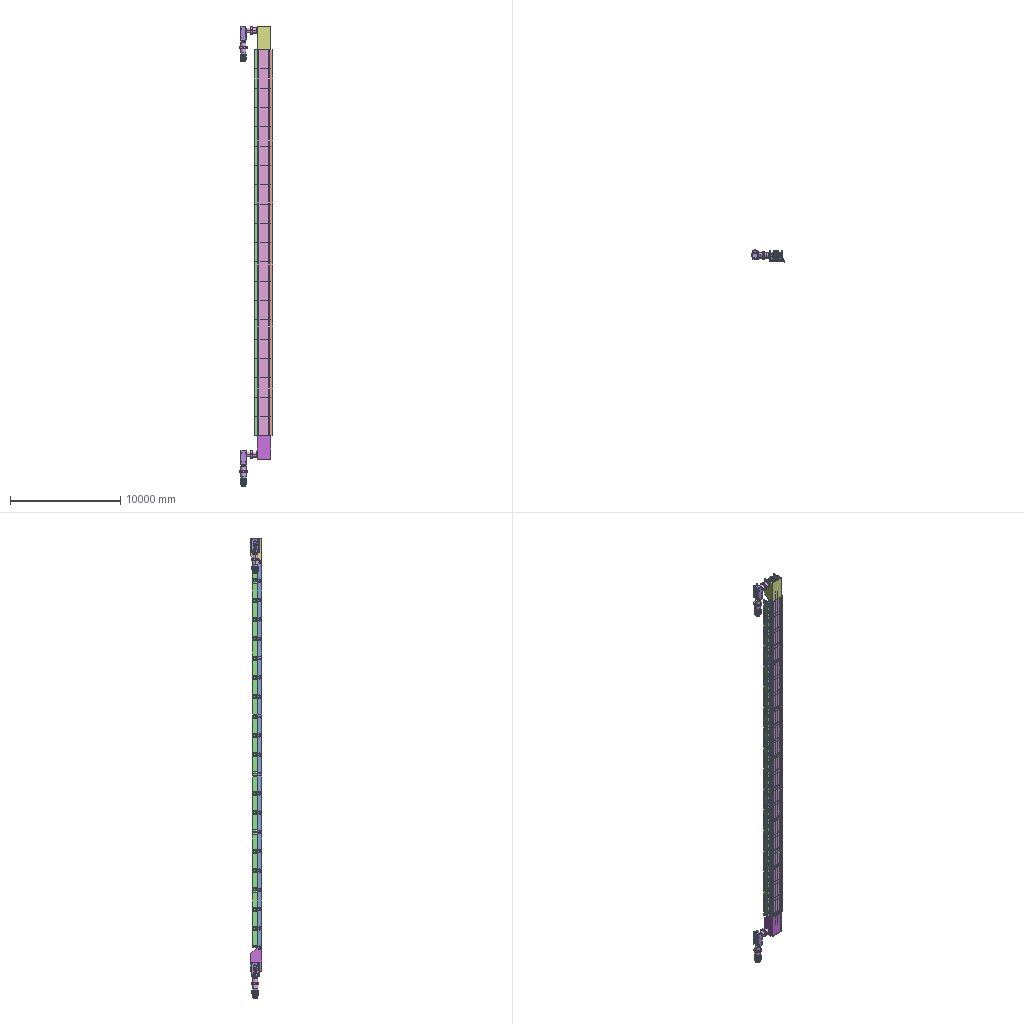Assembly | SolidWorks | 41 different items | 1422 placed | box 2996 x 1048 x 41686 mm
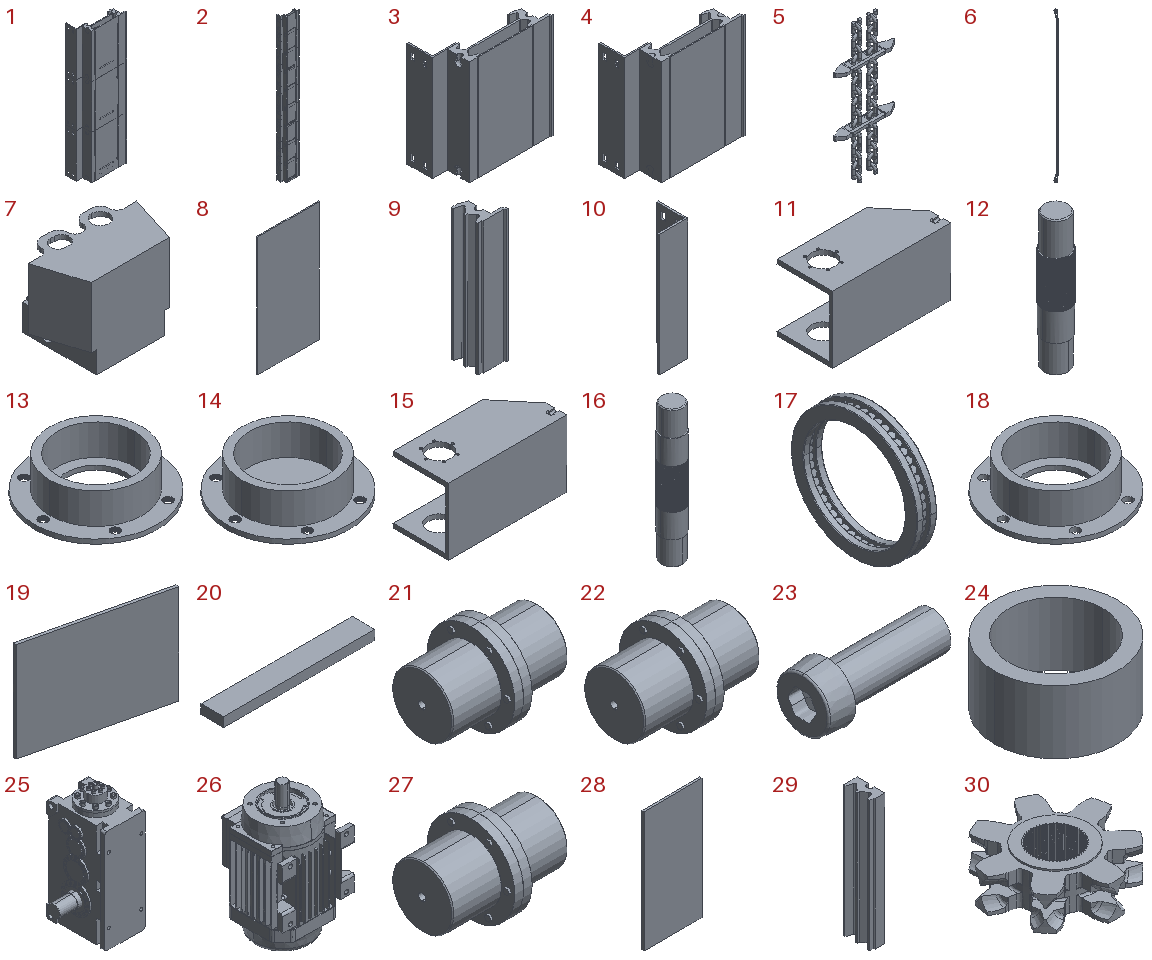Parts list (item | name | quantity | parent item | size | volume | features):
1 | (subassembly) | x6 | in 2 | 1628 x 811.488 x 5250 mm | 1041325350 mm3 | -
2 | (subassembly) | x2 | - | - | 3123900816 mm3 | -
3 | (subassembly) | x1 | - | 1628 x 811.488 x 1750 mm | 332107465 mm3 | -
4 | (subassembly) | x20 | in 1 | 1628 x 811.488 x 1750 mm | 345627340 mm3 | -
5 | (subassembly) | x1 | - | 984.376 x 173.983 x 2274 mm | 39316055 mm3 | features ReferencePattern 36, Cut 1, LocalChainPattern 1
6 | (subassembly) | x2 | - | - | 584235551 mm3 | features ReferencePattern 518, RefAxis 2, LocalChainPattern 1
7 | - | x40 | in 4 | 498.198 x 340 x 380 mm | 18859661 mm3 | features ICE 7, 3DProfileFeature 6, BlendCut 1, Extrusion 1, MirrorPattern 1
8 | - | x20 | in 4 | 903 x 15 x 1750 mm | 23703750 mm3 | features Extrusion 1
9 | - | x20 | in 4 | 368.945 x 388.507 x 1750 mm | 104894918 mm3 | features 3DProfileFeature 2, ICE 2, Extrusion 1, MirrorPattern 1, RevCut 1
10 | - | x20 | in 4 | 410 x 422.981 x 1750 mm | 34749166 mm3 | features Extrusion 1, ICE 1
11 | - | x1 | - | 2125 x 1000 x 1200 mm | 401885685 mm3 | features ICE 6, 3DProfileFeature 4, MirrorPattern 4, Extrusion 1, RevCut 1
12 | - | x1 | - | 294.723 x 294.709 x 1450 mm | 87344155 mm3 | features ICE 5, 3DProfileFeature 1, Chamfer 1, CirPattern 1, Extrusion 1, Fillet 1
13 | - | x1 | - | 560 x 560 x 160 mm | 9604413 mm3 | features SweepThread 6, ICE 4, 3DProfileFeature 1, Extrusion 1
14 | - | x1 | - | 560 x 560 x 160 mm | 10700722 mm3 | features SweepThread 6, ICE 3, 3DProfileFeature 1, Extrusion 1
15 | - | x1 | - | 2125 x 1000 x 1200 mm | 401885685 mm3 | features ICE 6, 3DProfileFeature 4, MirrorPattern 4, Extrusion 1, RevCut 1
16 | - | x1 | - | 294.723 x 294.709 x 1700 mm | 103257734 mm3 | features ICE 7, 3DProfileFeature 1, Chamfer 1, CirPattern 1, Extrusion 1, Fillet 1
17 | - | x1 | - | 53 x 350 x 350 mm | 1385597 mm3 | features Revolution 3, CirPattern 1, Fillet 1
18 | - | x1 | - | 560 x 560 x 160 mm | 9598744 mm3 | features ICE 4, 3DProfileFeature 1, Extrusion 1
19 | - | x2 | - | 1325 x 345 x 1000 mm | 39735000 mm3 | features Extrusion 1
20 | - | x1 | - | 800 x 120 x 50 mm | 4800000 mm3 | features Extrusion 1
21 | - | x1 | - | 605 x 460 x 460 mm | 55419022 mm3 | features ICE 15, Chamfer 6, Revolution 3, CirPattern 2, Fillet 2
22 | - | x4 | - | 907.5 x 690 x 690 mm | 187039199 mm3 | features ICE 15, Chamfer 6, Revolution 3, CirPattern 2, Fillet 2, Scale 1
23 | - | x1 | - | 115.6 x 51 x 51 mm | 120826 mm3 | features BlendCut 1, Cut 1, Extrusion 1, Fillet 1, LPattern 1, RevCut 1, Revolution 1, Scale 1
24 | - | x4 | - | 420 x 420 x 216 mm | 12553804 mm3 | features Extrusion 1, ICE 1
25 | - | x2 | - | 763.452 x 810 x 1512 mm | 419343636 mm3 | features MBimport 1, Scale 1
26 | - | x2 | - | 540 x 615 x 978 mm | 147963352 mm3 | features ICE 38, Fillet 18, MirrorPattern 10, Extrusion 5, CirPattern 4, Revolution 4, LibraryFeature 3, Chamfer 2, Dome 2, LPattern 2, CombineBodies 1, Scale 1, Shell 1
27 | - | x1 | - | 423.5 x 322 x 322 mm | 19008725 mm3 | features ICE 15, Chamfer 6, Revolution 3, CirPattern 2, Fillet 2, Scale 1
28 | - | x20 | in 4 | 840.28 x 30 x 1750 mm | 44114700 mm3 | features Extrusion 1
29 | - | x20 | in 4 | 187.997 x 370.453 x 1750 mm | 86925596 mm3 | features 3DProfileFeature 1, Extrusion 1, ICE 1, MirrorPattern 1, RevCut 1
30 | - | x4 | in 6 | 777.762 x 761.728 x 244 mm | 45916773 mm3 | features ICE 8, CirPattern 6, Fillet 3, MirrorPattern 2, 3DProfileFeature 1, BlendCut 1, Extrusion 1
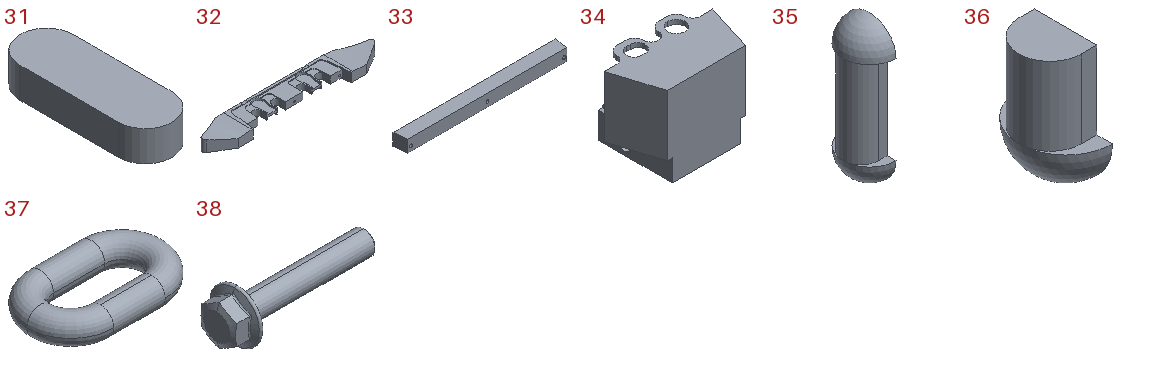31 | - | x2 | - | 56 x 160 x 32 mm | 265184 mm3 | features Extrusion 1
32 | - | x48 | in 1, 4 | 984.004 x 165 x 67.16 mm | 4451171 mm3 | features MirrorPattern 11, ICE 9, 3DProfileFeature 4, Extrusion 1
33 | - | x40 | in 4 | 550.66 x 45.55 x 40.5 mm | 995279 mm3 | features Extrusion 1, ICE 1
34 | - | x1 | - | 498.198 x 340 x 380 mm | 18832693 mm3 | features ICE 7, 3DProfileFeature 6, BlendCut 1, Extrusion 1, MirrorPattern 1
35 | - | x1 | - | 60 x 120 x 320 mm | 1275044 mm3 | features 3DProfileFeature 1, Extrusion 1, MirrorPattern 1, Revolution 1
36 | - | x84 | in 4 | 60 x 120 x 160 mm | 637522 mm3 | features 3DProfileFeature 1, Extrusion 1, Revolution 1
37 | - | x1040 | in 6 | 248 x 156 x 48 mm | 946927 mm3 | features Sweep 1
38 | - | x1 | - | 64.2 x 22.3 x 22.3 mm | 6417 mm3 | features Fillet 2, RevCut 2, Boss 1, Chamfer 1, Extrusion 1, LPattern 1, Revolution 1
39 | cylindrical thrust roller bearings gb | x1 | - | - | - | -
40 | hex flange bolts-heavy grade b gb | x1 | - | - | - | -
41 | hex lobular socket head cap screws-4.8 gb | x1 | - | - | - | -
Mates (type | each side: item.copy, entity, surface, feature):
In the top assembly
Coincident | 8.1 face plane Boss-Extrude 1 | 8.2 face plane Boss-Extrude 1
Coincident | 9.1 face plane Boss-Extrude 1 | 9.2 face plane Boss-Extrude 1
Coincident | 28.1 face plane Boss-Extrude 1 | 28.2 face plane Boss-Extrude 1
Coincident | 28.3 face plane Boss-Extrude 1 | 28.4 face plane Boss-Extrude 1
Coincident | 8.3 face plane Boss-Extrude 1 | 8.4 face plane Boss-Extrude 1
Coincident | 9.3 face plane Boss-Extrude 1 | 9.4 face plane Boss-Extrude 1
Coincident | 28.5 face plane Boss-Extrude 1 | 28.4 face plane Boss-Extrude 1
Coincident | 8.5 face plane Boss-Extrude 1 | 8.4 face plane Boss-Extrude 1
Coincident | 9.5 face plane Boss-Extrude 1 | 9.4 face plane Boss-Extrude 1
Coincident | 15.1 face plane Mirror 5 | 19.1 face plane Boss-Extrude 1 | 2 times
Coincident | 19.1 face plane Boss-Extrude 1 | 15.1 face plane Boss-Extrude 4
Coincident | 11.1 face plane Boss-Extrude 4 | 19.2 face plane Boss-Extrude 1 | 3 times
Concentric | 11.1 face cylinder Cut-Extrude 3 | 14.1 face cylinder Boss-Extrude 2
Coincident | 11.1 face plane Boss-Extrude 3 | 14.1 face plane Boss-Extrude 1
Concentric | 11.1 face cylinder Cut-Extrude 3 | 13.1 face cylinder Boss-Extrude 2
Coincident | 11.1 face plane Boss-Extrude 1 | 13.1 face plane Boss-Extrude 1
Concentric | 15.1 face cylinder Cut-Extrude 3 | 18.1 face cylinder Boss-Extrude 2
Coincident | 15.1 face plane Boss-Extrude 3 | 18.1 face plane Boss-Extrude 1
Coincident | 28.6 face plane Boss-Extrude 1 | 15.1 face plane Boss-Extrude 1
Coincident | 29.1 face plane Boss-Extrude 1 | 15.1 face plane Boss-Extrude 1
Coincident | 29.1 edge | 15.1 edge
Coincident | 28.1 face plane Boss-Extrude 1 | 11.1 face plane Boss-Extrude 1
Coincident | 29.2 edge | 11.1 edge
Coincident | 29.2 face plane Boss-Extrude 1 | 11.1 face plane Boss-Extrude 1
Coincident | assembly edge | assembly edge | 2 times
Concentric | assembly edge | assembly edge | 2 times
Concentric | 13.1 face cylinder Cut-Extrude 1 | 24.1 face cylinder Boss-Extrude 1
Concentric | 18.1 face cylinder Cut-Extrude 1 | assembly edge
Coincident | assembly face | 24.2 face plane Boss-Extrude 1
Coincident | 13.1 face plane Boss-Extrude 2 | 24.1 face plane Boss-Extrude 1
Coincident | assembly face | 24.3 face plane Boss-Extrude 1
Concentric | 25.1 face cylinder MR3[MR3-1-A-45-Ⅰ-E-JB╱ZQ6101-2002].step | 26.1 face cylinder Revolve 1
Parallel | 25.1 face plane MR3[MR3-1-A-45-Ⅰ-E-JB╱ZQ6101-2002].step | 26.1 face plane Boss-Extrude 13
Concentric | 25.2 face cylinder MR3[MR3-1-A-45-Ⅰ-E-JB╱ZQ6101-2002].step | 26.2 face cylinder Revolve 1
Parallel | 25.2 face plane MR3[MR3-1-A-45-Ⅰ-E-JB╱ZQ6101-2002].step | 26.2 face plane Mirror 9
Concentric | 25.1 face cylinder MR3[MR3-1-A-45-Ⅰ-E-JB╱ZQ6101-2002].step | 22.1 face cylinder Revolve 1
Coincident | 26.1 face plane Revolve 2 | 22.1 face plane Revolve 2
Coincident | 25.1 face plane MR3[MR3-1-A-45-Ⅰ-E-JB╱ZQ6101-2002].step | 22.1 face plane Revolve 1
Parallel | 15.1 face plane Boss-Extrude 1 | 25.1 face plane MR3[MR3-1-A-45-Ⅰ-E-JB╱ZQ6101-2002].step
Concentric | 25.2 face cylinder MR3[MR3-1-A-45-Ⅰ-E-JB╱ZQ6101-2002].step | 22.2 face cylinder Revolve 1
Coincident | 26.2 face plane Revolve 2 | 22.2 face plane Revolve 2
Coincident | 25.2 face plane MR3[MR3-1-A-45-Ⅰ-E-JB╱ZQ6101-2002].step | 22.2 face plane Revolve 1
Parallel | 11.1 face plane Boss-Extrude 1 | 25.2 face plane MR3[MR3-1-A-45-Ⅰ-E-JB╱ZQ6101-2002].step
Coincident | 25.2 face plane MR3[MR3-1-A-45-Ⅰ-E-JB╱ZQ6101-2002].step | assembly face
Coincident | assembly face | assembly face | 2 times
Concentric | 14.1 face cylinder Cut-Extrude 2 | assembly face
Concentric | 13.1 face cylinder Cut-Extrude 1 | assembly face
Concentric | 18.1 face cylinder Cut-Extrude 1 | assembly face
Concentric | 13.1 face cylinder Cut-Extrude 1 | 12.1 face
Coincident | assembly face | 12.1 face plane Boss-Extrude 1
Coincident | 24.4 face plane Boss-Extrude 1 | assembly face
Concentric | 18.1 face cylinder Boss-Extrude 2 | 24.2 face cylinder Boss-Extrude 1
Coincident | 18.1 face plane Boss-Extrude 2 | 24.2 face plane Boss-Extrude 1
Concentric | 24.3 face cylinder Boss-Extrude 1 | 12.1 face
Coincident | 14.1 face plane Boss-Extrude 2 | 24.3 face plane Boss-Extrude 1
Concentric | 24.1 face cylinder Boss-Extrude 1 | 12.1 face
Concentric | assembly face | 12.1 face
Concentric | 25.2 face cylinder MR3[MR3-1-A-45-Ⅰ-E-JB╱ZQ6101-2002].step | 12.1 face
Concentric | 12.1 face | 22.3 face cylinder Revolve 2
Tangent | 15.1 face cylinder Mirror 6 | 18.1 edge
Perpendicular | 15.1 face plane Boss-Extrude 3 | 22.4 face plane Cut-Extrude 10
Coincident | 25.1 face plane MR3[MR3-1-A-45-Ⅰ-E-JB╱ZQ6101-2002].step | 22.4 face plane Revolve 1
Coincident | 25.2 edge | 22.3 face plane Revolve 1
Perpendicular | 11.1 face plane Boss-Extrude 1 | 22.3 face plane Cut-Extrude 10
Parallel | 12.1 face | 22.3 face plane Cut-Extrude 10
Tangent | 12.1 face | 31.1 face plane Boss-Extrude 1
Coincident | 12.1 face | 31.1 face plane Boss-Extrude 1
Tangent | 12.1 face | 31.1 face cylinder Boss-Extrude 1
Coincident | 15.1 face plane Boss-Extrude 3 | 36.1 face plane Boss-Extrude 1
Coincident | 15.1 face plane Cut-Extrude 6 | 36.1 edge
Coincident | 15.1 face plane Boss-Extrude 1 | 36.1 face plane Boss-Extrude 1
Coincident | 15.1 face plane Mirror 7 | 36.2 face plane Boss-Extrude 1
Coincident | 15.1 face plane Boss-Extrude 1 | 36.2 face plane Boss-Extrude 1 | 2 times
Coincident | 11.1 edge | 36.3 face plane Boss-Extrude 1
Coincident | 11.1 face plane Boss-Extrude 3 | 36.3 face plane Boss-Extrude 1
Coincident | 11.1 face plane Boss-Extrude 1 | 36.3 face plane Boss-Extrude 1
Coincident | 11.1 face plane Boss-Extrude 1 | 36.4 face plane Boss-Extrude 1 | 2 times
Coincident | 11.1 face plane Mirror 7 | 36.4 face plane Boss-Extrude 1
Coincident | 30.1 face plane Boss-Extrude 4 | 30.2 face plane Boss-Extrude 4
Concentric | 30.1 face cylinder Boss-Extrude 4 | 30.2 face cylinder Boss-Extrude 4
Coincident | 24.4 face plane Boss-Extrude 1 | 30.1 face plane Boss-Extrude 4
Coincident | 30.3 face plane Boss-Extrude 4 | 30.4 face plane Boss-Extrude 4
Concentric | 30.3 face cylinder Boss-Extrude 4 | 30.4 face cylinder Boss-Extrude 4
Coincident | 24.1 face plane Boss-Extrude 1 | 30.4 edge
Concentric | 24.1 face cylinder Boss-Extrude 1 | 30.4 edge
Coincident | 32.1 face plane Boss-Extrude 1 | 28.1 face plane Boss-Extrude 1
Coincident | 28.6 face plane Boss-Extrude 1 | 32.2 face plane Boss-Extrude 1
Concentric | 32.2 face cylinder Mirror 3 | assembly face
Coincident | 32.2 face plane Boss-Extrude 1 | assembly face | 3 times
Concentric | 32.2 face cylinder Cut-Extrude 1 | assembly face | 2 times
Concentric | 32.1 face cylinder Mirror 3 | assembly face
Coincident | 32.1 face plane Boss-Extrude 1 | assembly face | 3 times
Concentric | 32.1 face cylinder Cut-Extrude 1 | assembly face | 2 times
In subassembly 6
Coincident | 30.5 plane | 6.1 plane
Coincident | 30.6 plane | 6.1 plane
Concentric | 30.6 face cylinder Boss-Extrude 4 | 6.1 axis
Concentric | 30.5 face cylinder Boss-Extrude 4 | 6.1 axis
In subassembly 2
Coincident | 9.6 face plane Boss-Extrude 1 | 9.7 face plane Boss-Extrude 1 | 3 times
Coincident | 9.8 face plane Boss-Extrude 1 | 9.9 face plane Boss-Extrude 1 | 2 times
Coincident | 9.10 face plane Boss-Extrude 1 | 9.9 face plane Boss-Extrude 1
In subassembly 1
Coincident | 29.3 face plane Boss-Extrude 1 | 29.4 face plane Boss-Extrude 1 | 3 times
Coincident | 29.2 face plane Boss-Extrude 1 | 29.3 face plane Boss-Extrude 1 | 3 times
Coincident | 28.1 face plane Boss-Extrude 1 | 32.1 face plane Boss-Extrude 1
In subassembly 4
Coincident | 9.11 face plane Boss-Extrude 1 | 28.7 face plane Boss-Extrude 1 | 4 times
Coincident | 29.5 face plane Boss-Extrude 1 | 28.7 face plane Boss-Extrude 1 | 3 times
Coincident | 29.5 face plane Boss-Extrude 1 | 8.6 face plane Boss-Extrude 1 | 2 times
Coincident | 28.7 face plane Boss-Extrude 1 | 32.1 face plane Boss-Extrude 1
Coincident | 8.6 face plane Boss-Extrude 1 | 32.2 face plane Boss-Extrude 1
Coincident | 9.11 face plane Cut-Extrude 2 | 36.2 face plane Boss-Extrude 1
Coincident | 9.11 face plane Boss-Extrude 1 | 36.2 face plane Boss-Extrude 1 | 2 times
Coincident | 9.11 face plane Boss-Extrude 1 | 36.3 face plane Boss-Extrude 1 | 2 times
Coincident | 9.11 face plane Mirror 1 | 36.3 face plane Boss-Extrude 1
Coincident | 29.5 face plane Boss-Extrude 1 | 36.4 face plane Boss-Extrude 1 | 2 times
Coincident | 29.5 face plane Cut-Extrude 3 | 36.4 face plane Boss-Extrude 1
Coincident | 29.5 face plane Boss-Extrude 1 | 36.1 face plane Boss-Extrude 1 | 2 times
Coincident | 29.5 edge | 36.1 face plane Boss-Extrude 1
Concentric | 32.1 face cylinder Mirror 3 | 4.1 face
Coincident | 32.1 face plane Boss-Extrude 1 | 4.1 face
Coincident | 29.5 face plane Boss-Extrude 1 | 10.1 face plane Boss-Extrude 1 | 2 times
Coincident | 7.1 face plane Boss-Extrude 4 | 10.1 face plane Boss-Extrude 1
Coincident | 7.1 face plane Boss-Extrude 2 | 10.1 face plane Boss-Extrude 1
Coincident | 7.2 face plane Boss-Extrude 4 | 10.1 face plane Boss-Extrude 1
Coincident | 7.2 face plane Boss-Extrude 2 | 10.1 face plane Boss-Extrude 1
Coincident | 32.1 face plane Cut-Extrude 17 | 33.1 face plane Boss-Extrude 1
Coincident | 32.1 face plane Cut-Extrude 6 | 33.1 face plane Boss-Extrude 1
Coincident | 32.1 edge | 33.1 edge
Coincident | 32.2 face plane Cut-Extrude 17 | 33.2 face plane Boss-Extrude 1
Coincident | 32.2 face plane Cut-Extrude 6 | 33.2 face plane Boss-Extrude 1
Coincident | 32.2 edge | 33.2 edge